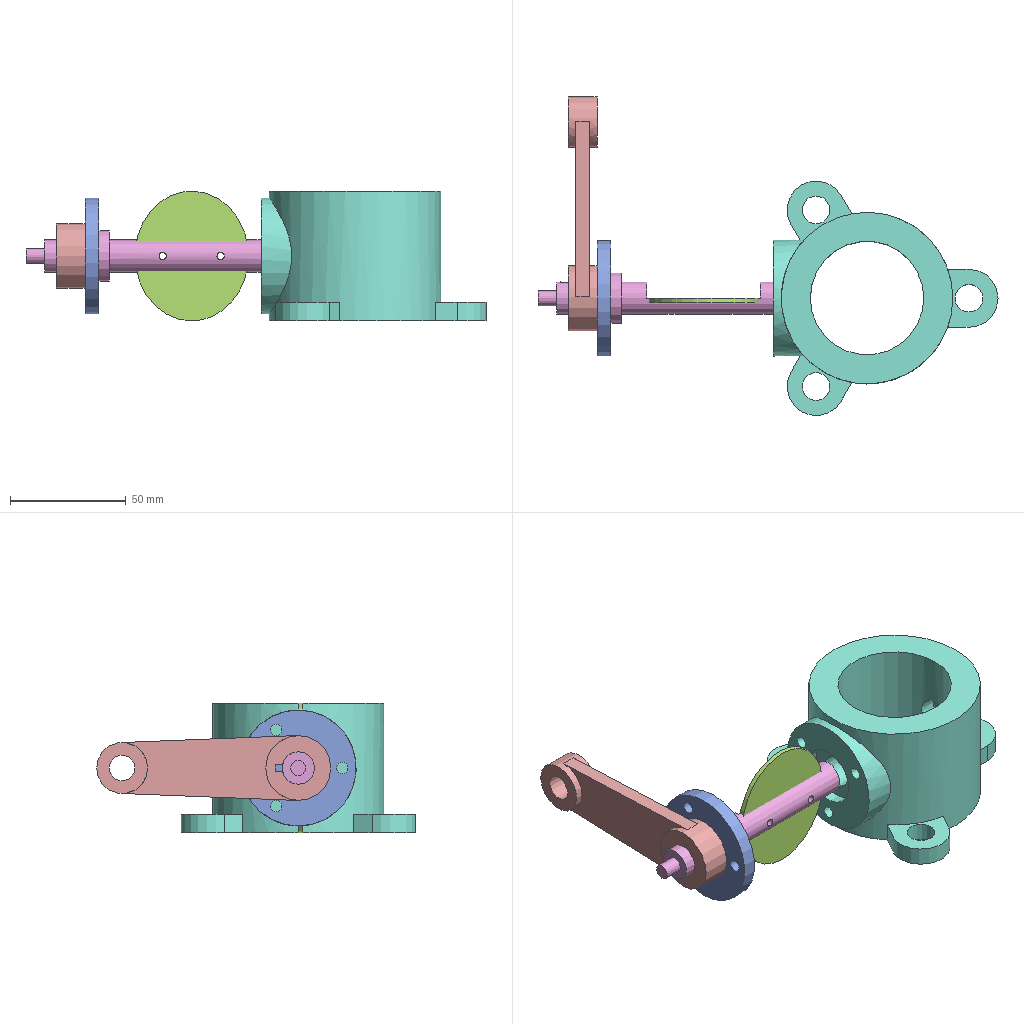Assembly | NX | 10 different items | 10 placed | box 198 x 138 x 56 mm
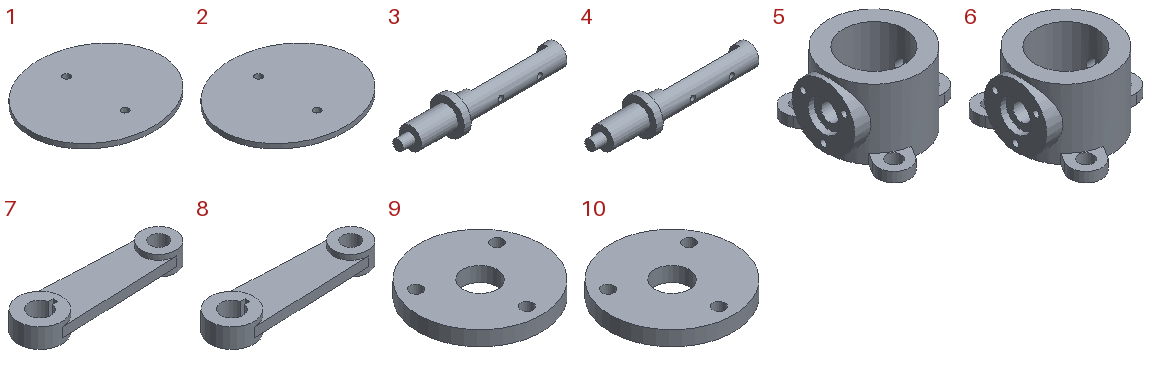Parts list (item | quantity | size | volume | features):
1 | x1 | 56 x 49 x 2 mm | 4282 mm3 | features DATUM_CSYS 2, EXTRUDE 1, SKETCH 1
2 | x1 | 56 x 49 x 2 mm | 4282 mm3 | features DATUM_CSYS 2, EXTRUDE 1, SKETCH 1
3 | x1 | 101.5 x 22 x 22 mm | 11635 mm3 | features DATUM_CSYS 5, SKETCH 4, EXTRUDE 3, SWP104 1
4 | x1 | 101.5 x 22 x 22 mm | 11635 mm3 | features DATUM_CSYS 5, SKETCH 4, EXTRUDE 3, SWP104 1
5 | x1 | 97 x 101.21 x 56 mm | 148727 mm3 | features DATUM_CSYS 8, EXTRUDE 7, SKETCH 7
6 | x1 | 97 x 101.21 x 56 mm | 148727 mm3 | features DATUM_CSYS 8, EXTRUDE 7, SKETCH 7
7 | x1 | 101 x 28 x 12.5 mm | 17643 mm3 | features EXTRUDE 3, DATUM_CSYS 2, SKETCH 1
8 | x1 | 101 x 28 x 12.5 mm | 17643 mm3 | features EXTRUDE 3, DATUM_CSYS 2, SKETCH 1
9 | x1 | 50 x 50 x 6 mm | 10504 mm3 | features DATUM_CSYS 2, EXTRUDE 1, SKETCH 1
10 | x1 | 50 x 50 x 6 mm | 10504 mm3 | features DATUM_CSYS 2, EXTRUDE 1, SKETCH 1
Mates (type | each side: item.copy, entity, surface, feature):
Fix | 5.1 component
Touch | 9.1 face plane Extrude(2) | 3.1 face plane Revolve(2)
Touch | 7.1 face plane Extrude(2) | 9.1 face plane Extrude(2)
Concentric | 1.1 edge | 3.1 arc
Concentric | 3.1 edge | 5.1 edge